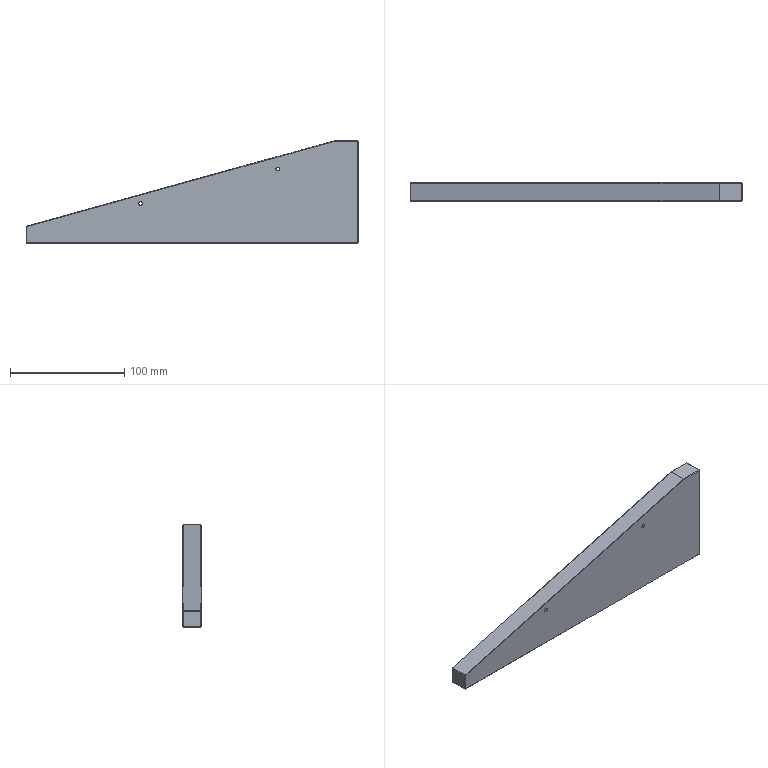Part | STEP file | ND25021-01-JDKM-04-TL | 1 solid | 53 faces | box 290 x 16 x 90 mm | volume 253250 mm3 | plane 29 | cylinder 14 | cone 10 | commonest cylinder face diameters 5 x10 3.3 x4